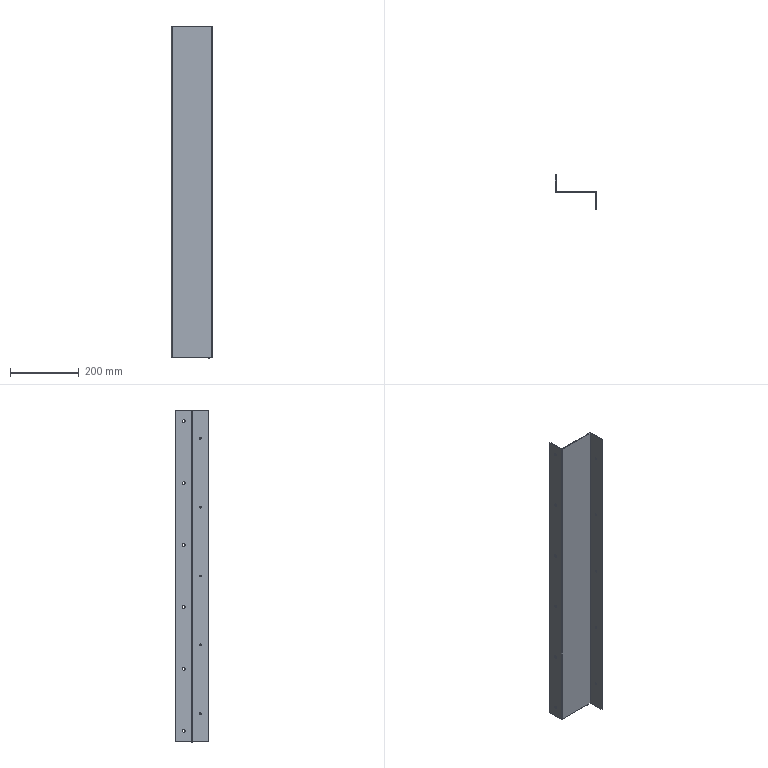Part | STEP file | SX-006-02 | 1 solid | 52 faces | box 120 x 98 x 965.5 mm | volume 412579 mm3 | cylinder 26 | plane 26 | commonest cylinder face diameters 8 x12 5.4 x10 0.4 x2 4.4 x2